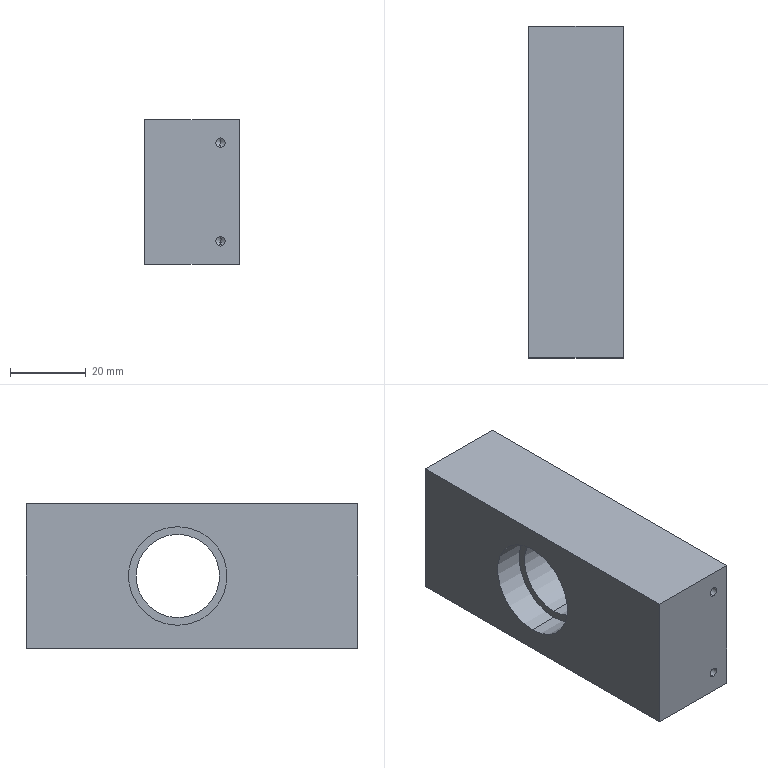Part | STEP file | 0243_217_Housing | 1 solid | 38 faces | box 25 x 87.5 x 38 mm | volume 70422 mm3 | cylinder 18 | cone 12 | plane 8 | commonest cylinder face diameters 4.2 x8 2.5 x4 26 x4 22 x2